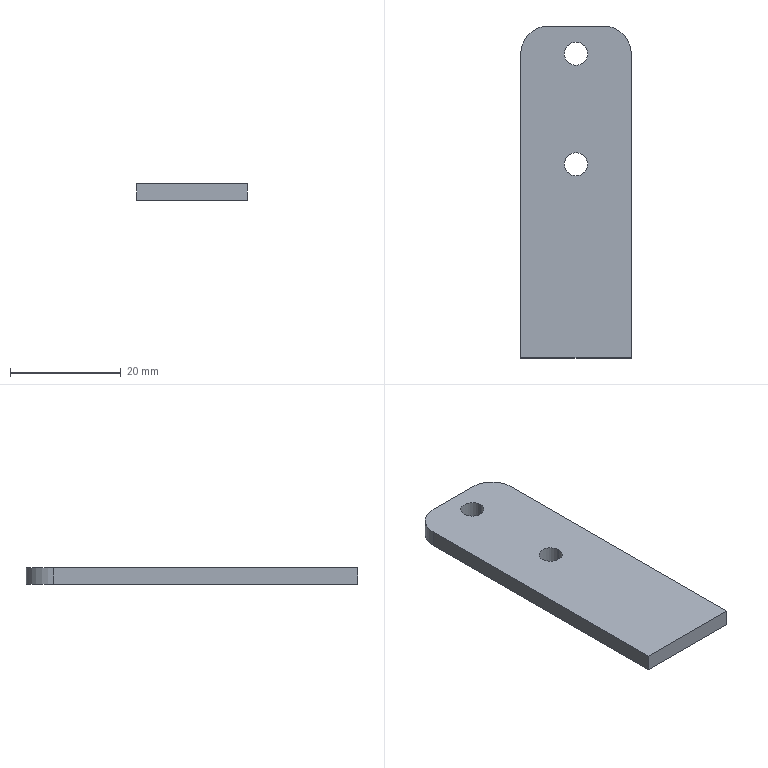Part | 1 solid | 12 faces | box 20 x 60 x 3 mm | volume 3485 mm3 | cylinder 6 | plane 6 | commonest cylinder face diameters 4.2 x4 10 x2
STEP:
#1=CARTESIAN_POINT('',(-2.1,25.,-3.));
#2=VERTEX_POINT('',#1);
#3=CARTESIAN_POINT('',(2.1,25.,-3.));
#4=VERTEX_POINT('',#3);
#5=CARTESIAN_POINT('',(0.,25.,-3.));
#6=DIRECTION('',(0.,0.,1.));
#7=DIRECTION('',(1.,0.,0.));
#8=AXIS2_PLACEMENT_3D('',#5,#6,#7);
#9=CIRCLE('',#8,2.1);
#10=EDGE_CURVE('',#2,#4,#9,.T.);
#11=ORIENTED_EDGE('',*,*,#10,.F.);
#12=CARTESIAN_POINT('',(-2.1,25.,0.));
#13=VERTEX_POINT('',#12);
#14=CARTESIAN_POINT('',(-2.1,25.,0.));
#15=DIRECTION('',(0.,0.,1.));
#16=VECTOR('',#15,1000.);
#17=LINE('',#14,#16);
#18=EDGE_CURVE('',#2,#13,#17,.T.);
#19=ORIENTED_EDGE('',*,*,#18,.T.);
#20=CARTESIAN_POINT('',(2.1,25.,0.));
#21=VERTEX_POINT('',#20);
#22=CARTESIAN_POINT('',(0.,25.,0.));
#23=DIRECTION('',(0.,0.,1.));
#24=DIRECTION('',(1.,0.,0.));
#25=AXIS2_PLACEMENT_3D('',#22,#23,#24);
#26=CIRCLE('',#25,2.1);
#27=EDGE_CURVE('',#13,#21,#26,.T.);
#28=ORIENTED_EDGE('',*,*,#27,.T.);
#29=CARTESIAN_POINT('',(2.1,25.,0.));
#30=DIRECTION('',(0.,0.,1.));
#31=VECTOR('',#30,1000.);
#32=LINE('',#29,#31);
#33=EDGE_CURVE('',#4,#21,#32,.T.);
#34=ORIENTED_EDGE('',*,*,#33,.F.);
#35=EDGE_LOOP('',(#11,#19,#28,#34));
#36=FACE_OUTER_BOUND('',#35,.T.);
#37=CARTESIAN_POINT('',(0.,25.,0.));
#38=DIRECTION('',(0.,0.,1.));
#39=DIRECTION('',(1.,0.,0.));
#40=AXIS2_PLACEMENT_3D('',#37,#38,#39);
#41=CYLINDRICAL_SURFACE('',#40,2.1);
#42=ADVANCED_FACE('',(#36),#41,.F.);
#43=CARTESIAN_POINT('',(-2.1,5.,-3.));
#44=VERTEX_POINT('',#43);
#45=CARTESIAN_POINT('',(2.1,5.,-3.));
#46=VERTEX_POINT('',#45);
#47=CARTESIAN_POINT('',(0.,5.,-3.));
#48=DIRECTION('',(0.,0.,1.));
#49=DIRECTION('',(1.,0.,0.));
#50=AXIS2_PLACEMENT_3D('',#47,#48,#49);
#51=CIRCLE('',#50,2.1);
#52=EDGE_CURVE('',#44,#46,#51,.T.);
#53=ORIENTED_EDGE('',*,*,#52,.F.);
#54=CARTESIAN_POINT('',(-2.1,5.,0.));
#55=VERTEX_POINT('',#54);
#56=CARTESIAN_POINT('',(-2.1,5.,0.));
#57=DIRECTION('',(0.,0.,1.));
#58=VECTOR('',#57,1000.);
#59=LINE('',#56,#58);
#60=EDGE_CURVE('',#44,#55,#59,.T.);
#61=ORIENTED_EDGE('',*,*,#60,.T.);
#62=CARTESIAN_POINT('',(2.1,5.,0.));
#63=VERTEX_POINT('',#62);
#64=CARTESIAN_POINT('',(0.,5.,0.));
#65=DIRECTION('',(0.,0.,1.));
#66=DIRECTION('',(1.,0.,0.));
#67=AXIS2_PLACEMENT_3D('',#64,#65,#66);
#68=CIRCLE('',#67,2.1);
#69=EDGE_CURVE('',#55,#63,#68,.T.);
#70=ORIENTED_EDGE('',*,*,#69,.T.);
#71=CARTESIAN_POINT('',(2.1,5.,0.));
#72=DIRECTION('',(0.,0.,1.));
#73=VECTOR('',#72,1000.);
#74=LINE('',#71,#73);
#75=EDGE_CURVE('',#46,#63,#74,.T.);
#76=ORIENTED_EDGE('',*,*,#75,.F.);
#77=EDGE_LOOP('',(#53,#61,#70,#76));
#78=FACE_OUTER_BOUND('',#77,.T.);
#79=CARTESIAN_POINT('',(0.,5.,0.));
#80=DIRECTION('',(0.,0.,1.));
#81=DIRECTION('',(1.,0.,0.));
#82=AXIS2_PLACEMENT_3D('',#79,#80,#81);
#83=CYLINDRICAL_SURFACE('',#82,2.1);
#84=ADVANCED_FACE('',(#78),#83,.F.);
#85=CARTESIAN_POINT('',(10.,-30.,0.));
#86=VERTEX_POINT('',#85);
#87=CARTESIAN_POINT('',(10.,25.,0.));
#88=VERTEX_POINT('',#87);
#89=CARTESIAN_POINT('',(10.,25.,0.));
#90=DIRECTION('',(0.,1.,0.));
#91=VECTOR('',#90,1000.);
#92=LINE('',#89,#91);
#93=EDGE_CURVE('',#86,#88,#92,.T.);
#94=ORIENTED_EDGE('',*,*,#93,.F.);
#95=CARTESIAN_POINT('',(10.,-30.,-3.));
#96=VERTEX_POINT('',#95);
#97=CARTESIAN_POINT('',(10.,-30.,-3.));
#98=DIRECTION('',(0.,0.,1.));
#99=VECTOR('',#98,1000.);
#100=LINE('',#97,#99);
#101=EDGE_CURVE('',#96,#86,#100,.T.);
#102=ORIENTED_EDGE('',*,*,#101,.F.);
#103=CARTESIAN_POINT('',(10.,25.,-3.));
#104=VERTEX_POINT('',#103);
#105=CARTESIAN_POINT('',(10.,25.,-3.));
#106=DIRECTION('',(0.,1.,0.));
#107=VECTOR('',#106,1000.);
#108=LINE('',#105,#107);
#109=EDGE_CURVE('',#96,#104,#108,.T.);
#110=ORIENTED_EDGE('',*,*,#109,.T.);
#111=CARTESIAN_POINT('',(10.,25.,-3.));
#112=DIRECTION('',(0.,0.,1.));
#113=VECTOR('',#112,1000.);
#114=LINE('',#111,#113);
#115=EDGE_CURVE('',#104,#88,#114,.T.);
#116=ORIENTED_EDGE('',*,*,#115,.T.);
#117=EDGE_LOOP('',(#94,#102,#110,#116));
#118=FACE_OUTER_BOUND('',#117,.T.);
#119=CARTESIAN_POINT('',(10.,25.,-3.));
#120=DIRECTION('',(1.,0.,0.));
#121=DIRECTION('',(0.,1.,0.));
#122=AXIS2_PLACEMENT_3D('',#119,#120,#121);
#123=PLANE('',#122);
#124=ADVANCED_FACE('',(#118),#123,.T.);
#125=CARTESIAN_POINT('',(-10.,-30.,0.));
#126=VERTEX_POINT('',#125);
#127=CARTESIAN_POINT('',(-10.,-30.,0.));
#128=DIRECTION('',(1.,0.,0.));
#129=VECTOR('',#128,1000.);
#130=LINE('',#127,#129);
#131=EDGE_CURVE('',#126,#86,#130,.T.);
#132=ORIENTED_EDGE('',*,*,#131,.F.);
#133=CARTESIAN_POINT('',(-10.,-30.,-3.));
#134=VERTEX_POINT('',#133);
#135=CARTESIAN_POINT('',(-10.,-30.,-3.));
#136=DIRECTION('',(0.,0.,1.));
#137=VECTOR('',#136,1000.);
#138=LINE('',#135,#137);
#139=EDGE_CURVE('',#134,#126,#138,.T.);
#140=ORIENTED_EDGE('',*,*,#139,.F.);
#141=CARTESIAN_POINT('',(-10.,-30.,-3.));
#142=DIRECTION('',(1.,0.,0.));
#143=VECTOR('',#142,1000.);
#144=LINE('',#141,#143);
#145=EDGE_CURVE('',#134,#96,#144,.T.);
#146=ORIENTED_EDGE('',*,*,#145,.T.);
#147=ORIENTED_EDGE('',*,*,#101,.T.);
#148=EDGE_LOOP('',(#132,#140,#146,#147));
#149=FACE_OUTER_BOUND('',#148,.T.);
#150=CARTESIAN_POINT('',(-10.,-30.,-3.));
#151=DIRECTION('',(0.,-1.,0.));
#152=DIRECTION('',(0.,0.,-1.));
#153=AXIS2_PLACEMENT_3D('',#150,#151,#152);
#154=PLANE('',#153);
#155=ADVANCED_FACE('',(#149),#154,.T.);
#156=CARTESIAN_POINT('',(-10.,25.,0.));
#157=VERTEX_POINT('',#156);
#158=CARTESIAN_POINT('',(-10.,25.,0.));
#159=DIRECTION('',(0.,-1.,0.));
#160=VECTOR('',#159,1000.);
#161=LINE('',#158,#160);
#162=EDGE_CURVE('',#157,#126,#161,.T.);
#163=ORIENTED_EDGE('',*,*,#162,.F.);
#164=CARTESIAN_POINT('',(-10.,25.,-3.));
#165=VERTEX_POINT('',#164);
#166=CARTESIAN_POINT('',(-10.,25.,-3.));
#167=DIRECTION('',(0.,0.,1.));
#168=VECTOR('',#167,1000.);
#169=LINE('',#166,#168);
#170=EDGE_CURVE('',#165,#157,#169,.T.);
#171=ORIENTED_EDGE('',*,*,#170,.F.);
#172=CARTESIAN_POINT('',(-10.,25.,-3.));
#173=DIRECTION('',(0.,-1.,0.));
#174=VECTOR('',#173,1000.);
#175=LINE('',#172,#174);
#176=EDGE_CURVE('',#165,#134,#175,.T.);
#177=ORIENTED_EDGE('',*,*,#176,.T.);
#178=ORIENTED_EDGE('',*,*,#139,.T.);
#179=EDGE_LOOP('',(#163,#171,#177,#178));
#180=FACE_OUTER_BOUND('',#179,.T.);
#181=CARTESIAN_POINT('',(-10.,25.,-3.));
#182=DIRECTION('',(-1.,0.,0.));
#183=DIRECTION('',(0.,-1.,0.));
#184=AXIS2_PLACEMENT_3D('',#181,#182,#183);
#185=PLANE('',#184);
#186=ADVANCED_FACE('',(#180),#185,.T.);
#187=CARTESIAN_POINT('',(-5.,30.,0.));
#188=VERTEX_POINT('',#187);
#189=CARTESIAN_POINT('',(-5.,25.,0.));
#190=DIRECTION('',(0.,0.,1.));
#191=DIRECTION('',(1.,0.,0.));
#192=AXIS2_PLACEMENT_3D('',#189,#190,#191);
#193=CIRCLE('',#192,5.);
#194=EDGE_CURVE('',#188,#157,#193,.T.);
#195=ORIENTED_EDGE('',*,*,#194,.F.);
#196=CARTESIAN_POINT('',(-5.,30.,-3.));
#197=VERTEX_POINT('',#196);
#198=CARTESIAN_POINT('',(-5.,30.,-3.));
#199=DIRECTION('',(0.,0.,1.));
#200=VECTOR('',#199,1000.);
#201=LINE('',#198,#200);
#202=EDGE_CURVE('',#197,#188,#201,.T.);
#203=ORIENTED_EDGE('',*,*,#202,.F.);
#204=CARTESIAN_POINT('',(-5.,25.,-3.));
#205=DIRECTION('',(0.,0.,1.));
#206=DIRECTION('',(1.,0.,0.));
#207=AXIS2_PLACEMENT_3D('',#204,#205,#206);
#208=CIRCLE('',#207,5.);
#209=EDGE_CURVE('',#197,#165,#208,.T.);
#210=ORIENTED_EDGE('',*,*,#209,.T.);
#211=ORIENTED_EDGE('',*,*,#170,.T.);
#212=EDGE_LOOP('',(#195,#203,#210,#211));
#213=FACE_OUTER_BOUND('',#212,.T.);
#214=CARTESIAN_POINT('',(-5.,25.,-3.));
#215=DIRECTION('',(0.,0.,1.));
#216=DIRECTION('',(1.,0.,0.));
#217=AXIS2_PLACEMENT_3D('',#214,#215,#216);
#218=CYLINDRICAL_SURFACE('',#217,5.);
#219=ADVANCED_FACE('',(#213),#218,.T.);
#220=CARTESIAN_POINT('',(5.,30.,0.));
#221=VERTEX_POINT('',#220);
#222=CARTESIAN_POINT('',(-5.,30.,0.));
#223=DIRECTION('',(-1.,0.,0.));
#224=VECTOR('',#223,1000.);
#225=LINE('',#222,#224);
#226=EDGE_CURVE('',#221,#188,#225,.T.);
#227=ORIENTED_EDGE('',*,*,#226,.F.);
#228=CARTESIAN_POINT('',(5.,30.,-3.));
#229=VERTEX_POINT('',#228);
#230=CARTESIAN_POINT('',(5.,30.,-3.));
#231=DIRECTION('',(0.,0.,1.));
#232=VECTOR('',#231,1000.);
#233=LINE('',#230,#232);
#234=EDGE_CURVE('',#229,#221,#233,.T.);
#235=ORIENTED_EDGE('',*,*,#234,.F.);
#236=CARTESIAN_POINT('',(-5.,30.,-3.));
#237=DIRECTION('',(-1.,0.,0.));
#238=VECTOR('',#237,1000.);
#239=LINE('',#236,#238);
#240=EDGE_CURVE('',#229,#197,#239,.T.);
#241=ORIENTED_EDGE('',*,*,#240,.T.);
#242=ORIENTED_EDGE('',*,*,#202,.T.);
#243=EDGE_LOOP('',(#227,#235,#241,#242));
#244=FACE_OUTER_BOUND('',#243,.T.);
#245=CARTESIAN_POINT('',(-5.,30.,-3.));
#246=DIRECTION('',(0.,1.,0.));
#247=DIRECTION('',(0.,0.,1.));
#248=AXIS2_PLACEMENT_3D('',#245,#246,#247);
#249=PLANE('',#248);
#250=ADVANCED_FACE('',(#244),#249,.T.);
#251=CARTESIAN_POINT('',(5.,25.,0.));
#252=DIRECTION('',(0.,0.,1.));
#253=DIRECTION('',(-1.,0.,0.));
#254=AXIS2_PLACEMENT_3D('',#251,#252,#253);
#255=CIRCLE('',#254,5.);
#256=EDGE_CURVE('',#88,#221,#255,.T.);
#257=ORIENTED_EDGE('',*,*,#256,.F.);
#258=ORIENTED_EDGE('',*,*,#115,.F.);
#259=CARTESIAN_POINT('',(5.,25.,-3.));
#260=DIRECTION('',(0.,0.,1.));
#261=DIRECTION('',(-1.,0.,0.));
#262=AXIS2_PLACEMENT_3D('',#259,#260,#261);
#263=CIRCLE('',#262,5.);
#264=EDGE_CURVE('',#104,#229,#263,.T.);
#265=ORIENTED_EDGE('',*,*,#264,.T.);
#266=ORIENTED_EDGE('',*,*,#234,.T.);
#267=EDGE_LOOP('',(#257,#258,#265,#266));
#268=FACE_OUTER_BOUND('',#267,.T.);
#269=CARTESIAN_POINT('',(5.,25.,-3.));
#270=DIRECTION('',(0.,0.,1.));
#271=DIRECTION('',(1.,0.,0.));
#272=AXIS2_PLACEMENT_3D('',#269,#270,#271);
#273=CYLINDRICAL_SURFACE('',#272,5.);
#274=ADVANCED_FACE('',(#268),#273,.T.);
#275=CARTESIAN_POINT('',(0.,25.,-3.));
#276=DIRECTION('',(0.,0.,1.));
#277=DIRECTION('',(1.,0.,0.));
#278=AXIS2_PLACEMENT_3D('',#275,#276,#277);
#279=CIRCLE('',#278,2.1);
#280=EDGE_CURVE('',#4,#2,#279,.T.);
#281=ORIENTED_EDGE('',*,*,#280,.T.);
#282=ORIENTED_EDGE('',*,*,#10,.T.);
#283=EDGE_LOOP('',(#281,#282));
#284=FACE_BOUND('',#283,.T.);
#285=CARTESIAN_POINT('',(0.,5.,-3.));
#286=DIRECTION('',(0.,0.,1.));
#287=DIRECTION('',(1.,0.,0.));
#288=AXIS2_PLACEMENT_3D('',#285,#286,#287);
#289=CIRCLE('',#288,2.1);
#290=EDGE_CURVE('',#46,#44,#289,.T.);
#291=ORIENTED_EDGE('',*,*,#290,.T.);
#292=ORIENTED_EDGE('',*,*,#52,.T.);
#293=EDGE_LOOP('',(#291,#292));
#294=FACE_BOUND('',#293,.T.);
#295=ORIENTED_EDGE('',*,*,#109,.F.);
#296=ORIENTED_EDGE('',*,*,#145,.F.);
#297=ORIENTED_EDGE('',*,*,#176,.F.);
#298=ORIENTED_EDGE('',*,*,#209,.F.);
#299=ORIENTED_EDGE('',*,*,#240,.F.);
#300=ORIENTED_EDGE('',*,*,#264,.F.);
#301=EDGE_LOOP('',(#295,#296,#297,#298,#299,#300));
#302=FACE_OUTER_BOUND('',#301,.T.);
#303=CARTESIAN_POINT('',(-5.,25.,-3.));
#304=DIRECTION('',(0.,0.,1.));
#305=DIRECTION('',(1.,0.,0.));
#306=AXIS2_PLACEMENT_3D('',#303,#304,#305);
#307=PLANE('',#306);
#308=ADVANCED_FACE('',(#284,#294,#302),#307,.F.);
#309=CARTESIAN_POINT('',(0.,25.,0.));
#310=DIRECTION('',(0.,0.,1.));
#311=DIRECTION('',(1.,0.,0.));
#312=AXIS2_PLACEMENT_3D('',#309,#310,#311);
#313=CIRCLE('',#312,2.1);
#314=EDGE_CURVE('',#21,#13,#313,.T.);
#315=ORIENTED_EDGE('',*,*,#314,.F.);
#316=ORIENTED_EDGE('',*,*,#27,.F.);
#317=EDGE_LOOP('',(#315,#316));
#318=FACE_BOUND('',#317,.T.);
#319=CARTESIAN_POINT('',(0.,5.,0.));
#320=DIRECTION('',(0.,0.,1.));
#321=DIRECTION('',(1.,0.,0.));
#322=AXIS2_PLACEMENT_3D('',#319,#320,#321);
#323=CIRCLE('',#322,2.1);
#324=EDGE_CURVE('',#63,#55,#323,.T.);
#325=ORIENTED_EDGE('',*,*,#324,.F.);
#326=ORIENTED_EDGE('',*,*,#69,.F.);
#327=EDGE_LOOP('',(#325,#326));
#328=FACE_BOUND('',#327,.T.);
#329=ORIENTED_EDGE('',*,*,#93,.T.);
#330=ORIENTED_EDGE('',*,*,#256,.T.);
#331=ORIENTED_EDGE('',*,*,#226,.T.);
#332=ORIENTED_EDGE('',*,*,#194,.T.);
#333=ORIENTED_EDGE('',*,*,#162,.T.);
#334=ORIENTED_EDGE('',*,*,#131,.T.);
#335=EDGE_LOOP('',(#329,#330,#331,#332,#333,#334));
#336=FACE_OUTER_BOUND('',#335,.T.);
#337=CARTESIAN_POINT('',(-5.,25.,0.));
#338=DIRECTION('',(0.,0.,1.));
#339=DIRECTION('',(1.,0.,0.));
#340=AXIS2_PLACEMENT_3D('',#337,#338,#339);
#341=PLANE('',#340);
#342=ADVANCED_FACE('',(#318,#328,#336),#341,.T.);
#343=ORIENTED_EDGE('',*,*,#60,.F.);
#344=ORIENTED_EDGE('',*,*,#290,.F.);
#345=ORIENTED_EDGE('',*,*,#75,.T.);
#346=ORIENTED_EDGE('',*,*,#324,.T.);
#347=EDGE_LOOP('',(#343,#344,#345,#346));
#348=FACE_OUTER_BOUND('',#347,.T.);
#349=CARTESIAN_POINT('',(0.,5.,0.));
#350=DIRECTION('',(0.,0.,1.));
#351=DIRECTION('',(1.,0.,0.));
#352=AXIS2_PLACEMENT_3D('',#349,#350,#351);
#353=CYLINDRICAL_SURFACE('',#352,2.1);
#354=ADVANCED_FACE('',(#348),#353,.F.);
#355=ORIENTED_EDGE('',*,*,#18,.F.);
#356=ORIENTED_EDGE('',*,*,#280,.F.);
#357=ORIENTED_EDGE('',*,*,#33,.T.);
#358=ORIENTED_EDGE('',*,*,#314,.T.);
#359=EDGE_LOOP('',(#355,#356,#357,#358));
#360=FACE_OUTER_BOUND('',#359,.T.);
#361=CARTESIAN_POINT('',(0.,25.,0.));
#362=DIRECTION('',(0.,0.,1.));
#363=DIRECTION('',(1.,0.,0.));
#364=AXIS2_PLACEMENT_3D('',#361,#362,#363);
#365=CYLINDRICAL_SURFACE('',#364,2.1);
#366=ADVANCED_FACE('',(#360),#365,.F.);
#367=CLOSED_SHELL('',(#42,#84,#124,#155,#186,#219,#250,#274,#308,#342,#354,#366));
#368=MANIFOLD_SOLID_BREP('',#367);
#369=CARTESIAN_POINT('',(0.,0.,0.));
#370=DIRECTION('',(0.,0.,1.));
#371=DIRECTION('',(1.,0.,0.));
#372=AXIS2_PLACEMENT_3D('',#369,#370,#371);
#373=(LENGTH_UNIT()NAMED_UNIT(*)SI_UNIT(.MILLI.,.METRE.));
#374=UNCERTAINTY_MEASURE_WITH_UNIT(LENGTH_MEASURE(0.00001),#373,'','');
#375=(NAMED_UNIT(*)PLANE_ANGLE_UNIT()SI_UNIT($,.RADIAN.));
#376=(NAMED_UNIT(*)SI_UNIT($,.STERADIAN.)SOLID_ANGLE_UNIT());
#377=(GEOMETRIC_REPRESENTATION_CONTEXT(3)GLOBAL_UNCERTAINTY_ASSIGNED_CONTEXT((#374))GLOBAL_UNIT_ASSIGNED_CONTEXT((#373,#375,#376))REPRESENTATION_CONTEXT('',''));
#378=ADVANCED_BREP_SHAPE_REPRESENTATION('',(#368,#372),#377);